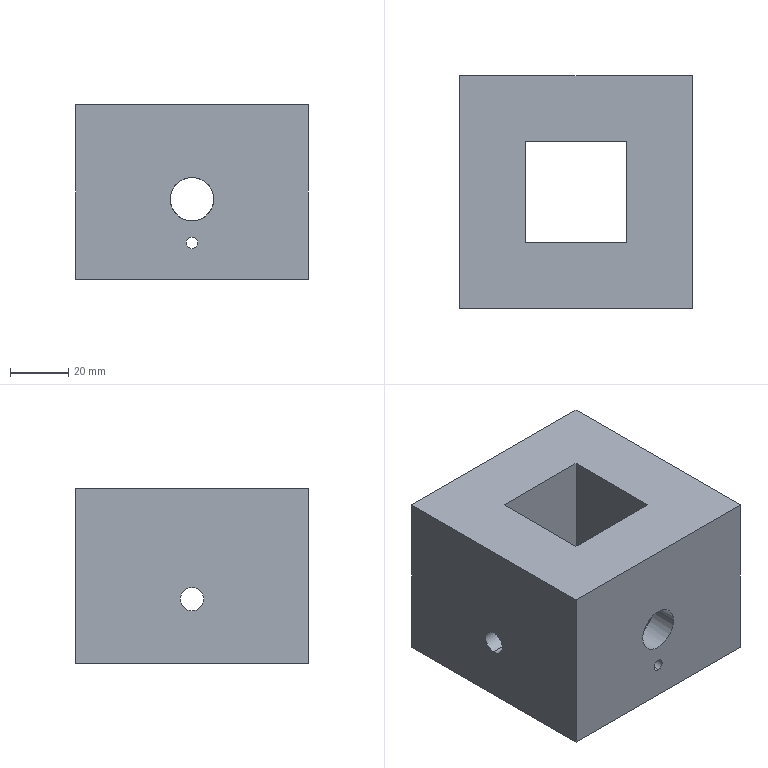Part | SolidWorks | features Cut 6, ICE 3, Extrusion 1 | 1 solid | 43 faces | box 80 x 80 x 60 mm | volume 271765 mm3 | plane 31 | cylinder 12 | commonest cylinder face diameters 4 x4 8 x4 15 x4
STEP:
#1=CARTESIAN_POINT('',(-91.5,-49.,10.5));
#2=VERTEX_POINT('',#1);
#3=CARTESIAN_POINT('',(-91.5,-49.,14.5));
#4=VERTEX_POINT('',#3);
#5=CARTESIAN_POINT('',(-91.5,-49.,12.5));
#6=DIRECTION('',(0.,1.,0.));
#7=DIRECTION('',(0.,0.,-1.));
#8=AXIS2_PLACEMENT_3D('',#5,#6,#7);
#9=CIRCLE('',#8,2.);
#10=EDGE_CURVE('',#2,#4,#9,.T.);
#11=ORIENTED_EDGE('',*,*,#10,.T.);
#12=CARTESIAN_POINT('',(-91.5,-61.5,14.5));
#13=VERTEX_POINT('',#12);
#14=CARTESIAN_POINT('',(-91.5,18.5,14.5));
#15=DIRECTION('',(0.,-1.,0.));
#16=VECTOR('',#15,1000.);
#17=LINE('',#14,#16);
#18=EDGE_CURVE('',#4,#13,#17,.T.);
#19=ORIENTED_EDGE('',*,*,#18,.T.);
#20=CARTESIAN_POINT('',(-91.5,-61.5,10.5));
#21=VERTEX_POINT('',#20);
#22=CARTESIAN_POINT('',(-91.5,-61.5,12.5));
#23=DIRECTION('',(0.,-1.,0.));
#24=DIRECTION('',(-1.,0.,0.));
#25=AXIS2_PLACEMENT_3D('',#22,#23,#24);
#26=CIRCLE('',#25,2.);
#27=EDGE_CURVE('',#13,#21,#26,.T.);
#28=ORIENTED_EDGE('',*,*,#27,.T.);
#29=CARTESIAN_POINT('',(-91.5,18.5,10.5));
#30=DIRECTION('',(0.,-1.,0.));
#31=VECTOR('',#30,1000.);
#32=LINE('',#29,#31);
#33=EDGE_CURVE('',#2,#21,#32,.T.);
#34=ORIENTED_EDGE('',*,*,#33,.F.);
#35=EDGE_LOOP('',(#11,#19,#28,#34));
#36=FACE_OUTER_BOUND('',#35,.T.);
#37=CARTESIAN_POINT('',(-91.5,18.5,12.5));
#38=DIRECTION('',(0.,-1.,0.));
#39=DIRECTION('',(0.,0.,-1.));
#40=AXIS2_PLACEMENT_3D('',#37,#38,#39);
#41=CYLINDRICAL_SURFACE('',#40,2.);
#42=ADVANCED_FACE('',(#36),#41,.F.);
#43=CARTESIAN_POINT('',(-91.5,18.5,10.5));
#44=VERTEX_POINT('',#43);
#45=CARTESIAN_POINT('',(-91.5,18.5,14.5));
#46=VERTEX_POINT('',#45);
#47=CARTESIAN_POINT('',(-91.5,18.5,12.5));
#48=DIRECTION('',(0.,1.,0.));
#49=DIRECTION('',(0.,0.,1.));
#50=AXIS2_PLACEMENT_3D('',#47,#48,#49);
#51=CIRCLE('',#50,2.);
#52=EDGE_CURVE('',#44,#46,#51,.T.);
#53=ORIENTED_EDGE('',*,*,#52,.T.);
#54=CARTESIAN_POINT('',(-91.5,6.,14.5));
#55=VERTEX_POINT('',#54);
#56=CARTESIAN_POINT('',(-91.5,18.5,14.5));
#57=DIRECTION('',(0.,-1.,0.));
#58=VECTOR('',#57,1000.);
#59=LINE('',#56,#58);
#60=EDGE_CURVE('',#46,#55,#59,.T.);
#61=ORIENTED_EDGE('',*,*,#60,.T.);
#62=CARTESIAN_POINT('',(-91.5,6.,10.5));
#63=VERTEX_POINT('',#62);
#64=CARTESIAN_POINT('',(-91.5,6.,12.5));
#65=DIRECTION('',(0.,-1.,0.));
#66=DIRECTION('',(0.,0.,1.));
#67=AXIS2_PLACEMENT_3D('',#64,#65,#66);
#68=CIRCLE('',#67,2.);
#69=EDGE_CURVE('',#55,#63,#68,.T.);
#70=ORIENTED_EDGE('',*,*,#69,.T.);
#71=CARTESIAN_POINT('',(-91.5,18.5,10.5));
#72=DIRECTION('',(0.,-1.,0.));
#73=VECTOR('',#72,1000.);
#74=LINE('',#71,#73);
#75=EDGE_CURVE('',#44,#63,#74,.T.);
#76=ORIENTED_EDGE('',*,*,#75,.F.);
#77=EDGE_LOOP('',(#53,#61,#70,#76));
#78=FACE_OUTER_BOUND('',#77,.T.);
#79=CARTESIAN_POINT('',(-91.5,18.5,12.5));
#80=DIRECTION('',(0.,-1.,0.));
#81=DIRECTION('',(0.,0.,-1.));
#82=AXIS2_PLACEMENT_3D('',#79,#80,#81);
#83=CYLINDRICAL_SURFACE('',#82,2.);
#84=ADVANCED_FACE('',(#78),#83,.F.);
#85=CARTESIAN_POINT('',(-51.5,-21.5,18.));
#86=VERTEX_POINT('',#85);
#87=CARTESIAN_POINT('',(-51.5,-21.5,26.));
#88=VERTEX_POINT('',#87);
#89=CARTESIAN_POINT('',(-51.5,-21.5,22.));
#90=DIRECTION('',(-1.,0.,0.));
#91=DIRECTION('',(0.,0.,1.));
#92=AXIS2_PLACEMENT_3D('',#89,#90,#91);
#93=CIRCLE('',#92,4.);
#94=EDGE_CURVE('',#86,#88,#93,.T.);
#95=ORIENTED_EDGE('',*,*,#94,.F.);
#96=CARTESIAN_POINT('',(-74.,-21.5,18.));
#97=VERTEX_POINT('',#96);
#98=CARTESIAN_POINT('',(-32.5,-21.5,18.));
#99=DIRECTION('',(-1.,0.,0.));
#100=VECTOR('',#99,1000.);
#101=LINE('',#98,#100);
#102=EDGE_CURVE('',#86,#97,#101,.T.);
#103=ORIENTED_EDGE('',*,*,#102,.T.);
#104=CARTESIAN_POINT('',(-74.,-21.5,26.));
#105=VERTEX_POINT('',#104);
#106=CARTESIAN_POINT('',(-74.,-21.5,22.));
#107=DIRECTION('',(1.,0.,0.));
#108=DIRECTION('',(0.,0.,-1.));
#109=AXIS2_PLACEMENT_3D('',#106,#107,#108);
#110=CIRCLE('',#109,4.);
#111=EDGE_CURVE('',#105,#97,#110,.T.);
#112=ORIENTED_EDGE('',*,*,#111,.F.);
#113=CARTESIAN_POINT('',(-32.5,-21.5,26.));
#114=DIRECTION('',(-1.,0.,0.));
#115=VECTOR('',#114,1000.);
#116=LINE('',#113,#115);
#117=EDGE_CURVE('',#88,#105,#116,.T.);
#118=ORIENTED_EDGE('',*,*,#117,.F.);
#119=EDGE_LOOP('',(#95,#103,#112,#118));
#120=FACE_OUTER_BOUND('',#119,.T.);
#121=CARTESIAN_POINT('',(-32.5,-21.5,22.));
#122=DIRECTION('',(-1.,0.,0.));
#123=DIRECTION('',(0.,0.,1.));
#124=AXIS2_PLACEMENT_3D('',#121,#122,#123);
#125=CYLINDRICAL_SURFACE('',#124,4.);
#126=ADVANCED_FACE('',(#120),#125,.F.);
#127=CARTESIAN_POINT('',(-109.,-21.5,18.));
#128=VERTEX_POINT('',#127);
#129=CARTESIAN_POINT('',(-109.,-21.5,26.));
#130=VERTEX_POINT('',#129);
#131=CARTESIAN_POINT('',(-109.,-21.5,22.));
#132=DIRECTION('',(-1.,0.,0.));
#133=DIRECTION('',(0.,0.,1.));
#134=AXIS2_PLACEMENT_3D('',#131,#132,#133);
#135=CIRCLE('',#134,4.);
#136=EDGE_CURVE('',#128,#130,#135,.T.);
#137=ORIENTED_EDGE('',*,*,#136,.F.);
#138=CARTESIAN_POINT('',(-131.5,-21.5,18.));
#139=VERTEX_POINT('',#138);
#140=CARTESIAN_POINT('',(-32.5,-21.5,18.));
#141=DIRECTION('',(-1.,0.,0.));
#142=VECTOR('',#141,1000.);
#143=LINE('',#140,#142);
#144=EDGE_CURVE('',#128,#139,#143,.T.);
#145=ORIENTED_EDGE('',*,*,#144,.T.);
#146=CARTESIAN_POINT('',(-131.5,-21.5,26.));
#147=VERTEX_POINT('',#146);
#148=CARTESIAN_POINT('',(-131.5,-21.5,22.));
#149=DIRECTION('',(-1.,0.,0.));
#150=DIRECTION('',(0.,0.,1.));
#151=AXIS2_PLACEMENT_3D('',#148,#149,#150);
#152=CIRCLE('',#151,4.);
#153=EDGE_CURVE('',#139,#147,#152,.T.);
#154=ORIENTED_EDGE('',*,*,#153,.T.);
#155=CARTESIAN_POINT('',(-32.5,-21.5,26.));
#156=DIRECTION('',(-1.,0.,0.));
#157=VECTOR('',#156,1000.);
#158=LINE('',#155,#157);
#159=EDGE_CURVE('',#130,#147,#158,.T.);
#160=ORIENTED_EDGE('',*,*,#159,.F.);
#161=EDGE_LOOP('',(#137,#145,#154,#160));
#162=FACE_OUTER_BOUND('',#161,.T.);
#163=CARTESIAN_POINT('',(-32.5,-21.5,22.));
#164=DIRECTION('',(-1.,0.,0.));
#165=DIRECTION('',(0.,0.,1.));
#166=AXIS2_PLACEMENT_3D('',#163,#164,#165);
#167=CYLINDRICAL_SURFACE('',#166,4.);
#168=ADVANCED_FACE('',(#162),#167,.F.);
#169=CARTESIAN_POINT('',(-91.5,8.5,20.));
#170=VERTEX_POINT('',#169);
#171=CARTESIAN_POINT('',(-99.,8.5,27.5));
#172=VERTEX_POINT('',#171);
#173=CARTESIAN_POINT('',(-91.5,8.5,27.5));
#174=DIRECTION('',(0.,1.,0.));
#175=DIRECTION('',(0.,0.,1.));
#176=AXIS2_PLACEMENT_3D('',#173,#174,#175);
#177=CIRCLE('',#176,7.5);
#178=EDGE_CURVE('',#170,#172,#177,.T.);
#179=ORIENTED_EDGE('',*,*,#178,.F.);
#180=CARTESIAN_POINT('',(-91.5,18.5,20.));
#181=VERTEX_POINT('',#180);
#182=CARTESIAN_POINT('',(-91.5,8.5,20.));
#183=DIRECTION('',(0.,1.,0.));
#184=VECTOR('',#183,1000.);
#185=LINE('',#182,#184);
#186=EDGE_CURVE('',#170,#181,#185,.T.);
#187=ORIENTED_EDGE('',*,*,#186,.T.);
#188=CARTESIAN_POINT('',(-91.5,18.5,35.));
#189=VERTEX_POINT('',#188);
#190=CARTESIAN_POINT('',(-91.5,18.5,27.5));
#191=DIRECTION('',(0.,1.,0.));
#192=DIRECTION('',(0.,0.,1.));
#193=AXIS2_PLACEMENT_3D('',#190,#191,#192);
#194=CIRCLE('',#193,7.5);
#195=EDGE_CURVE('',#181,#189,#194,.T.);
#196=ORIENTED_EDGE('',*,*,#195,.T.);
#197=CARTESIAN_POINT('',(-91.5,8.5,35.));
#198=VERTEX_POINT('',#197);
#199=CARTESIAN_POINT('',(-91.5,8.5,35.));
#200=DIRECTION('',(0.,1.,0.));
#201=VECTOR('',#200,1000.);
#202=LINE('',#199,#201);
#203=EDGE_CURVE('',#198,#189,#202,.T.);
#204=ORIENTED_EDGE('',*,*,#203,.F.);
#205=CARTESIAN_POINT('',(-91.5,8.5,27.5));
#206=DIRECTION('',(0.,1.,0.));
#207=DIRECTION('',(0.,0.,1.));
#208=AXIS2_PLACEMENT_3D('',#205,#206,#207);
#209=CIRCLE('',#208,7.5);
#210=EDGE_CURVE('',#172,#198,#209,.T.);
#211=ORIENTED_EDGE('',*,*,#210,.F.);
#212=EDGE_LOOP('',(#179,#187,#196,#204,#211));
#213=FACE_OUTER_BOUND('',#212,.T.);
#214=CARTESIAN_POINT('',(-91.5,8.5,27.5));
#215=DIRECTION('',(0.,1.,0.));
#216=DIRECTION('',(0.,0.,1.));
#217=AXIS2_PLACEMENT_3D('',#214,#215,#216);
#218=CYLINDRICAL_SURFACE('',#217,7.5);
#219=ADVANCED_FACE('',(#213),#218,.F.);
#220=CARTESIAN_POINT('',(-99.,-51.5,27.5));
#221=VERTEX_POINT('',#220);
#222=CARTESIAN_POINT('',(-91.5,-51.5,20.));
#223=VERTEX_POINT('',#222);
#224=CARTESIAN_POINT('',(-91.5,-51.5,27.5));
#225=DIRECTION('',(0.,-1.,0.));
#226=DIRECTION('',(1.,0.,0.));
#227=AXIS2_PLACEMENT_3D('',#224,#225,#226);
#228=CIRCLE('',#227,7.5);
#229=EDGE_CURVE('',#221,#223,#228,.T.);
#230=ORIENTED_EDGE('',*,*,#229,.F.);
#231=CARTESIAN_POINT('',(-99.,-61.5,27.5));
#232=VERTEX_POINT('',#231);
#233=CARTESIAN_POINT('',(-99.,-51.5,27.5));
#234=DIRECTION('',(0.,-1.,0.));
#235=VECTOR('',#234,1000.);
#236=LINE('',#233,#235);
#237=EDGE_CURVE('',#221,#232,#236,.T.);
#238=ORIENTED_EDGE('',*,*,#237,.T.);
#239=CARTESIAN_POINT('',(-84.,-61.5,27.5));
#240=VERTEX_POINT('',#239);
#241=CARTESIAN_POINT('',(-91.5,-61.5,27.5));
#242=DIRECTION('',(0.,-1.,0.));
#243=DIRECTION('',(1.,0.,0.));
#244=AXIS2_PLACEMENT_3D('',#241,#242,#243);
#245=CIRCLE('',#244,7.5);
#246=EDGE_CURVE('',#232,#240,#245,.T.);
#247=ORIENTED_EDGE('',*,*,#246,.T.);
#248=CARTESIAN_POINT('',(-84.,-51.5,27.5));
#249=VERTEX_POINT('',#248);
#250=CARTESIAN_POINT('',(-84.,-51.5,27.5));
#251=DIRECTION('',(0.,-1.,0.));
#252=VECTOR('',#251,1000.);
#253=LINE('',#250,#252);
#254=EDGE_CURVE('',#249,#240,#253,.T.);
#255=ORIENTED_EDGE('',*,*,#254,.F.);
#256=CARTESIAN_POINT('',(-91.5,-51.5,27.5));
#257=DIRECTION('',(0.,-1.,0.));
#258=DIRECTION('',(1.,0.,0.));
#259=AXIS2_PLACEMENT_3D('',#256,#257,#258);
#260=CIRCLE('',#259,7.5);
#261=EDGE_CURVE('',#223,#249,#260,.T.);
#262=ORIENTED_EDGE('',*,*,#261,.F.);
#263=EDGE_LOOP('',(#230,#238,#247,#255,#262));
#264=FACE_OUTER_BOUND('',#263,.T.);
#265=CARTESIAN_POINT('',(-91.5,-51.5,27.5));
#266=DIRECTION('',(0.,-1.,0.));
#267=DIRECTION('',(1.,0.,0.));
#268=AXIS2_PLACEMENT_3D('',#265,#266,#267);
#269=CYLINDRICAL_SURFACE('',#268,7.5);
#270=ADVANCED_FACE('',(#264),#269,.F.);
#271=CARTESIAN_POINT('',(-84.,8.5,27.5));
#272=VERTEX_POINT('',#271);
#273=CARTESIAN_POINT('',(-84.,8.5,35.));
#274=VERTEX_POINT('',#273);
#275=CARTESIAN_POINT('',(-84.,8.5,0.));
#276=DIRECTION('',(0.,0.,1.));
#277=VECTOR('',#276,1000.);
#278=LINE('',#275,#277);
#279=EDGE_CURVE('',#272,#274,#278,.T.);
#280=ORIENTED_EDGE('',*,*,#279,.F.);
#281=CARTESIAN_POINT('',(-84.,8.5,20.));
#282=VERTEX_POINT('',#281);
#283=CARTESIAN_POINT('',(-84.,8.5,0.));
#284=DIRECTION('',(0.,0.,1.));
#285=VECTOR('',#284,1000.);
#286=LINE('',#283,#285);
#287=EDGE_CURVE('',#282,#272,#286,.T.);
#288=ORIENTED_EDGE('',*,*,#287,.F.);
#289=CARTESIAN_POINT('',(-84.,-4.,20.));
#290=VERTEX_POINT('',#289);
#291=CARTESIAN_POINT('',(-84.,94.5,20.));
#292=DIRECTION('',(0.,-1.,0.));
#293=VECTOR('',#292,1000.);
#294=LINE('',#291,#293);
#295=EDGE_CURVE('',#282,#290,#294,.T.);
#296=ORIENTED_EDGE('',*,*,#295,.T.);
#297=CARTESIAN_POINT('',(-84.,-4.,35.));
#298=VERTEX_POINT('',#297);
#299=CARTESIAN_POINT('',(-84.,-4.,55.));
#300=DIRECTION('',(0.,0.,-1.));
#301=VECTOR('',#300,1000.);
#302=LINE('',#299,#301);
#303=EDGE_CURVE('',#298,#290,#302,.T.);
#304=ORIENTED_EDGE('',*,*,#303,.F.);
#305=CARTESIAN_POINT('',(-84.,94.5,35.));
#306=DIRECTION('',(0.,-1.,0.));
#307=VECTOR('',#306,1000.);
#308=LINE('',#305,#307);
#309=EDGE_CURVE('',#274,#298,#308,.T.);
#310=ORIENTED_EDGE('',*,*,#309,.F.);
#311=EDGE_LOOP('',(#280,#288,#296,#304,#310));
#312=FACE_OUTER_BOUND('',#311,.T.);
#313=CARTESIAN_POINT('',(-84.,94.5,20.));
#314=DIRECTION('',(1.,0.,0.));
#315=DIRECTION('',(0.,1.,0.));
#316=AXIS2_PLACEMENT_3D('',#313,#314,#315);
#317=PLANE('',#316);
#318=ADVANCED_FACE('',(#312),#317,.F.);
#319=CARTESIAN_POINT('',(0.,8.5,35.));
#320=DIRECTION('',(-1.,0.,0.));
#321=VECTOR('',#320,1000.);
#322=LINE('',#319,#321);
#323=EDGE_CURVE('',#274,#198,#322,.T.);
#324=ORIENTED_EDGE('',*,*,#323,.F.);
#325=ORIENTED_EDGE('',*,*,#309,.T.);
#326=CARTESIAN_POINT('',(-99.,-4.,35.));
#327=VERTEX_POINT('',#326);
#328=CARTESIAN_POINT('',(-74.,-4.,35.));
#329=DIRECTION('',(1.,0.,0.));
#330=VECTOR('',#329,1000.);
#331=LINE('',#328,#330);
#332=EDGE_CURVE('',#327,#298,#331,.T.);
#333=ORIENTED_EDGE('',*,*,#332,.F.);
#334=CARTESIAN_POINT('',(-99.,8.5,35.));
#335=VERTEX_POINT('',#334);
#336=CARTESIAN_POINT('',(-99.,94.5,35.));
#337=DIRECTION('',(0.,-1.,0.));
#338=VECTOR('',#337,1000.);
#339=LINE('',#336,#338);
#340=EDGE_CURVE('',#335,#327,#339,.T.);
#341=ORIENTED_EDGE('',*,*,#340,.F.);
#342=CARTESIAN_POINT('',(0.,8.5,35.));
#343=DIRECTION('',(-1.,0.,0.));
#344=VECTOR('',#343,1000.);
#345=LINE('',#342,#344);
#346=EDGE_CURVE('',#198,#335,#345,.T.);
#347=ORIENTED_EDGE('',*,*,#346,.F.);
#348=EDGE_LOOP('',(#324,#325,#333,#341,#347));
#349=FACE_OUTER_BOUND('',#348,.T.);
#350=CARTESIAN_POINT('',(-84.,94.5,35.));
#351=DIRECTION('',(0.,0.,1.));
#352=DIRECTION('',(1.,0.,0.));
#353=AXIS2_PLACEMENT_3D('',#350,#351,#352);
#354=PLANE('',#353);
#355=ADVANCED_FACE('',(#349),#354,.F.);
#356=CARTESIAN_POINT('',(-99.,8.5,0.));
#357=DIRECTION('',(0.,0.,-1.));
#358=VECTOR('',#357,1000.);
#359=LINE('',#356,#358);
#360=EDGE_CURVE('',#335,#172,#359,.T.);
#361=ORIENTED_EDGE('',*,*,#360,.F.);
#362=ORIENTED_EDGE('',*,*,#340,.T.);
#363=CARTESIAN_POINT('',(-99.,-4.,20.));
#364=VERTEX_POINT('',#363);
#365=CARTESIAN_POINT('',(-99.,-4.,55.));
#366=DIRECTION('',(0.,0.,1.));
#367=VECTOR('',#366,1000.);
#368=LINE('',#365,#367);
#369=EDGE_CURVE('',#364,#327,#368,.T.);
#370=ORIENTED_EDGE('',*,*,#369,.F.);
#371=CARTESIAN_POINT('',(-99.,8.5,20.));
#372=VERTEX_POINT('',#371);
#373=CARTESIAN_POINT('',(-99.,94.5,20.));
#374=DIRECTION('',(0.,-1.,0.));
#375=VECTOR('',#374,1000.);
#376=LINE('',#373,#375);
#377=EDGE_CURVE('',#372,#364,#376,.T.);
#378=ORIENTED_EDGE('',*,*,#377,.F.);
#379=CARTESIAN_POINT('',(-99.,8.5,0.));
#380=DIRECTION('',(0.,0.,-1.));
#381=VECTOR('',#380,1000.);
#382=LINE('',#379,#381);
#383=EDGE_CURVE('',#172,#372,#382,.T.);
#384=ORIENTED_EDGE('',*,*,#383,.F.);
#385=EDGE_LOOP('',(#361,#362,#370,#378,#384));
#386=FACE_OUTER_BOUND('',#385,.T.);
#387=CARTESIAN_POINT('',(-99.,94.5,20.));
#388=DIRECTION('',(-1.,0.,0.));
#389=DIRECTION('',(0.,-1.,0.));
#390=AXIS2_PLACEMENT_3D('',#387,#388,#389);
#391=PLANE('',#390);
#392=ADVANCED_FACE('',(#386),#391,.F.);
#393=CARTESIAN_POINT('',(0.,8.5,20.));
#394=DIRECTION('',(1.,0.,0.));
#395=VECTOR('',#394,1000.);
#396=LINE('',#393,#395);
#397=EDGE_CURVE('',#372,#170,#396,.T.);
#398=ORIENTED_EDGE('',*,*,#397,.F.);
#399=ORIENTED_EDGE('',*,*,#377,.T.);
#400=CARTESIAN_POINT('',(-74.,-4.,20.));
#401=DIRECTION('',(-1.,0.,0.));
#402=VECTOR('',#401,1000.);
#403=LINE('',#400,#402);
#404=EDGE_CURVE('',#290,#364,#403,.T.);
#405=ORIENTED_EDGE('',*,*,#404,.F.);
#406=ORIENTED_EDGE('',*,*,#295,.F.);
#407=CARTESIAN_POINT('',(0.,8.5,20.));
#408=DIRECTION('',(1.,0.,0.));
#409=VECTOR('',#408,1000.);
#410=LINE('',#407,#409);
#411=EDGE_CURVE('',#170,#282,#410,.T.);
#412=ORIENTED_EDGE('',*,*,#411,.F.);
#413=EDGE_LOOP('',(#398,#399,#405,#406,#412));
#414=FACE_OUTER_BOUND('',#413,.T.);
#415=CARTESIAN_POINT('',(-84.,94.5,20.));
#416=DIRECTION('',(0.,0.,-1.));
#417=DIRECTION('',(-1.,0.,0.));
#418=AXIS2_PLACEMENT_3D('',#415,#416,#417);
#419=PLANE('',#418);
#420=ADVANCED_FACE('',(#414),#419,.F.);
#421=CARTESIAN_POINT('',(-99.,-51.5,35.));
#422=VERTEX_POINT('',#421);
#423=CARTESIAN_POINT('',(-99.,-51.5,0.));
#424=DIRECTION('',(0.,0.,1.));
#425=VECTOR('',#424,1000.);
#426=LINE('',#423,#425);
#427=EDGE_CURVE('',#221,#422,#426,.T.);
#428=ORIENTED_EDGE('',*,*,#427,.F.);
#429=CARTESIAN_POINT('',(-99.,-51.5,20.));
#430=VERTEX_POINT('',#429);
#431=CARTESIAN_POINT('',(-99.,-51.5,0.));
#432=DIRECTION('',(0.,0.,1.));
#433=VECTOR('',#432,1000.);
#434=LINE('',#431,#433);
#435=EDGE_CURVE('',#430,#221,#434,.T.);
#436=ORIENTED_EDGE('',*,*,#435,.F.);
#437=CARTESIAN_POINT('',(-99.,-39.,20.));
#438=VERTEX_POINT('',#437);
#439=CARTESIAN_POINT('',(-99.,94.5,20.));
#440=DIRECTION('',(0.,-1.,0.));
#441=VECTOR('',#440,1000.);
#442=LINE('',#439,#441);
#443=EDGE_CURVE('',#438,#430,#442,.T.);
#444=ORIENTED_EDGE('',*,*,#443,.F.);
#445=CARTESIAN_POINT('',(-99.,-39.,35.));
#446=VERTEX_POINT('',#445);
#447=CARTESIAN_POINT('',(-99.,-39.,55.));
#448=DIRECTION('',(0.,0.,-1.));
#449=VECTOR('',#448,1000.);
#450=LINE('',#447,#449);
#451=EDGE_CURVE('',#446,#438,#450,.T.);
#452=ORIENTED_EDGE('',*,*,#451,.F.);
#453=CARTESIAN_POINT('',(-99.,94.5,35.));
#454=DIRECTION('',(0.,-1.,0.));
#455=VECTOR('',#454,1000.);
#456=LINE('',#453,#455);
#457=EDGE_CURVE('',#446,#422,#456,.T.);
#458=ORIENTED_EDGE('',*,*,#457,.T.);
#459=EDGE_LOOP('',(#428,#436,#444,#452,#458));
#460=FACE_OUTER_BOUND('',#459,.T.);
#461=CARTESIAN_POINT('',(-99.,94.5,20.));
#462=DIRECTION('',(-1.,0.,0.));
#463=DIRECTION('',(0.,-1.,0.));
#464=AXIS2_PLACEMENT_3D('',#461,#462,#463);
#465=PLANE('',#464);
#466=ADVANCED_FACE('',(#460),#465,.F.);
#467=CARTESIAN_POINT('',(-91.5,-51.5,35.));
#468=VERTEX_POINT('',#467);
#469=CARTESIAN_POINT('',(0.,-51.5,35.));
#470=DIRECTION('',(1.,0.,0.));
#471=VECTOR('',#470,1000.);
#472=LINE('',#469,#471);
#473=EDGE_CURVE('',#422,#468,#472,.T.);
#474=ORIENTED_EDGE('',*,*,#473,.F.);
#475=ORIENTED_EDGE('',*,*,#457,.F.);
#476=CARTESIAN_POINT('',(-84.,-39.,35.));
#477=VERTEX_POINT('',#476);
#478=CARTESIAN_POINT('',(-74.,-39.,35.));
#479=DIRECTION('',(-1.,0.,0.));
#480=VECTOR('',#479,1000.);
#481=LINE('',#478,#480);
#482=EDGE_CURVE('',#477,#446,#481,.T.);
#483=ORIENTED_EDGE('',*,*,#482,.F.);
#484=CARTESIAN_POINT('',(-84.,-51.5,35.));
#485=VERTEX_POINT('',#484);
#486=CARTESIAN_POINT('',(-84.,94.5,35.));
#487=DIRECTION('',(0.,-1.,0.));
#488=VECTOR('',#487,1000.);
#489=LINE('',#486,#488);
#490=EDGE_CURVE('',#477,#485,#489,.T.);
#491=ORIENTED_EDGE('',*,*,#490,.T.);
#492=CARTESIAN_POINT('',(0.,-51.5,35.));
#493=DIRECTION('',(1.,0.,0.));
#494=VECTOR('',#493,1000.);
#495=LINE('',#492,#494);
#496=EDGE_CURVE('',#468,#485,#495,.T.);
#497=ORIENTED_EDGE('',*,*,#496,.F.);
#498=EDGE_LOOP('',(#474,#475,#483,#491,#497));
#499=FACE_OUTER_BOUND('',#498,.T.);
#500=CARTESIAN_POINT('',(-84.,94.5,35.));
#501=DIRECTION('',(0.,0.,1.));
#502=DIRECTION('',(1.,0.,0.));
#503=AXIS2_PLACEMENT_3D('',#500,#501,#502);
#504=PLANE('',#503);
#505=ADVANCED_FACE('',(#499),#504,.F.);
#506=CARTESIAN_POINT('',(-84.,-51.5,0.));
#507=DIRECTION('',(0.,0.,-1.));
#508=VECTOR('',#507,1000.);
#509=LINE('',#506,#508);
#510=EDGE_CURVE('',#485,#249,#509,.T.);
#511=ORIENTED_EDGE('',*,*,#510,.F.);
#512=ORIENTED_EDGE('',*,*,#490,.F.);
#513=CARTESIAN_POINT('',(-84.,-39.,20.));
#514=VERTEX_POINT('',#513);
#515=CARTESIAN_POINT('',(-84.,-39.,55.));
#516=DIRECTION('',(0.,0.,1.));
#517=VECTOR('',#516,1000.);
#518=LINE('',#515,#517);
#519=EDGE_CURVE('',#514,#477,#518,.T.);
#520=ORIENTED_EDGE('',*,*,#519,.F.);
#521=CARTESIAN_POINT('',(-84.,-51.5,20.));
#522=VERTEX_POINT('',#521);
#523=CARTESIAN_POINT('',(-84.,94.5,20.));
#524=DIRECTION('',(0.,-1.,0.));
#525=VECTOR('',#524,1000.);
#526=LINE('',#523,#525);
#527=EDGE_CURVE('',#514,#522,#526,.T.);
#528=ORIENTED_EDGE('',*,*,#527,.T.);
#529=CARTESIAN_POINT('',(-84.,-51.5,0.));
#530=DIRECTION('',(0.,0.,-1.));
#531=VECTOR('',#530,1000.);
#532=LINE('',#529,#531);
#533=EDGE_CURVE('',#249,#522,#532,.T.);
#534=ORIENTED_EDGE('',*,*,#533,.F.);
#535=EDGE_LOOP('',(#511,#512,#520,#528,#534));
#536=FACE_OUTER_BOUND('',#535,.T.);
#537=CARTESIAN_POINT('',(-84.,94.5,20.));
#538=DIRECTION('',(1.,0.,0.));
#539=DIRECTION('',(0.,1.,0.));
#540=AXIS2_PLACEMENT_3D('',#537,#538,#539);
#541=PLANE('',#540);
#542=ADVANCED_FACE('',(#536),#541,.F.);
#543=CARTESIAN_POINT('',(0.,-51.5,20.));
#544=DIRECTION('',(-1.,0.,0.));
#545=VECTOR('',#544,1000.);
#546=LINE('',#543,#545);
#547=EDGE_CURVE('',#522,#223,#546,.T.);
#548=ORIENTED_EDGE('',*,*,#547,.F.);
#549=ORIENTED_EDGE('',*,*,#527,.F.);
#550=CARTESIAN_POINT('',(-74.,-39.,20.));
#551=DIRECTION('',(1.,0.,0.));
#552=VECTOR('',#551,1000.);
#553=LINE('',#550,#552);
#554=EDGE_CURVE('',#438,#514,#553,.T.);
#555=ORIENTED_EDGE('',*,*,#554,.F.);
#556=ORIENTED_EDGE('',*,*,#443,.T.);
#557=CARTESIAN_POINT('',(0.,-51.5,20.));
#558=DIRECTION('',(-1.,0.,0.));
#559=VECTOR('',#558,1000.);
#560=LINE('',#557,#559);
#561=EDGE_CURVE('',#223,#430,#560,.T.);
#562=ORIENTED_EDGE('',*,*,#561,.F.);
#563=EDGE_LOOP('',(#548,#549,#555,#556,#562));
#564=FACE_OUTER_BOUND('',#563,.T.);
#565=CARTESIAN_POINT('',(-84.,94.5,20.));
#566=DIRECTION('',(0.,0.,-1.));
#567=DIRECTION('',(-1.,0.,0.));
#568=AXIS2_PLACEMENT_3D('',#565,#566,#567);
#569=PLANE('',#568);
#570=ADVANCED_FACE('',(#564),#569,.F.);
#571=CARTESIAN_POINT('',(-131.5,-21.5,22.));
#572=DIRECTION('',(-1.,0.,0.));
#573=DIRECTION('',(0.,0.,1.));
#574=AXIS2_PLACEMENT_3D('',#571,#572,#573);
#575=CIRCLE('',#574,4.);
#576=EDGE_CURVE('',#147,#139,#575,.T.);
#577=ORIENTED_EDGE('',*,*,#576,.F.);
#578=ORIENTED_EDGE('',*,*,#153,.F.);
#579=EDGE_LOOP('',(#577,#578));
#580=FACE_BOUND('',#579,.T.);
#581=CARTESIAN_POINT('',(-131.5,18.5,60.));
#582=VERTEX_POINT('',#581);
#583=CARTESIAN_POINT('',(-131.5,18.5,0.));
#584=VERTEX_POINT('',#583);
#585=CARTESIAN_POINT('',(-131.5,18.5,60.));
#586=DIRECTION('',(0.,0.,-1.));
#587=VECTOR('',#586,1000.);
#588=LINE('',#585,#587);
#589=EDGE_CURVE('',#582,#584,#588,.T.);
#590=ORIENTED_EDGE('',*,*,#589,.T.);
#591=CARTESIAN_POINT('',(-131.5,-61.5,0.));
#592=VERTEX_POINT('',#591);
#593=CARTESIAN_POINT('',(-131.5,-61.5,0.));
#594=DIRECTION('',(0.,1.,0.));
#595=VECTOR('',#594,1000.);
#596=LINE('',#593,#595);
#597=EDGE_CURVE('',#592,#584,#596,.T.);
#598=ORIENTED_EDGE('',*,*,#597,.F.);
#599=CARTESIAN_POINT('',(-131.5,-61.5,60.));
#600=VERTEX_POINT('',#599);
#601=CARTESIAN_POINT('',(-131.5,-61.5,60.));
#602=DIRECTION('',(0.,0.,-1.));
#603=VECTOR('',#602,1000.);
#604=LINE('',#601,#603);
#605=EDGE_CURVE('',#600,#592,#604,.T.);
#606=ORIENTED_EDGE('',*,*,#605,.F.);
#607=CARTESIAN_POINT('',(-131.5,-61.5,60.));
#608=DIRECTION('',(0.,-1.,0.));
#609=VECTOR('',#608,1000.);
#610=LINE('',#607,#609);
#611=EDGE_CURVE('',#582,#600,#610,.T.);
#612=ORIENTED_EDGE('',*,*,#611,.F.);
#613=EDGE_LOOP('',(#590,#598,#606,#612));
#614=FACE_OUTER_BOUND('',#613,.T.);
#615=CARTESIAN_POINT('',(-131.5,-61.5,60.));
#616=DIRECTION('',(1.,0.,0.));
#617=DIRECTION('',(0.,0.,-1.));
#618=AXIS2_PLACEMENT_3D('',#615,#616,#617);
#619=PLANE('',#618);
#620=ADVANCED_FACE('',(#580,#614),#619,.F.);
#621=CARTESIAN_POINT('',(-91.5,-61.5,12.5));
#622=DIRECTION('',(0.,-1.,0.));
#623=DIRECTION('',(-1.,0.,0.));
#624=AXIS2_PLACEMENT_3D('',#621,#622,#623);
#625=CIRCLE('',#624,2.);
#626=EDGE_CURVE('',#21,#13,#625,.T.);
#627=ORIENTED_EDGE('',*,*,#626,.F.);
#628=ORIENTED_EDGE('',*,*,#27,.F.);
#629=EDGE_LOOP('',(#627,#628));
#630=FACE_BOUND('',#629,.T.);
#631=CARTESIAN_POINT('',(-91.5,-61.5,27.5));
#632=DIRECTION('',(0.,-1.,0.));
#633=DIRECTION('',(1.,0.,0.));
#634=AXIS2_PLACEMENT_3D('',#631,#632,#633);
#635=CIRCLE('',#634,7.5);
#636=EDGE_CURVE('',#240,#232,#635,.T.);
#637=ORIENTED_EDGE('',*,*,#636,.F.);
#638=ORIENTED_EDGE('',*,*,#246,.F.);
#639=EDGE_LOOP('',(#637,#638));
#640=FACE_BOUND('',#639,.T.);
#641=ORIENTED_EDGE('',*,*,#605,.T.);
#642=CARTESIAN_POINT('',(-51.5,-61.5,0.));
#643=VERTEX_POINT('',#642);
#644=CARTESIAN_POINT('',(-51.5,-61.5,0.));
#645=DIRECTION('',(-1.,0.,0.));
#646=VECTOR('',#645,1000.);
#647=LINE('',#644,#646);
#648=EDGE_CURVE('',#643,#592,#647,.T.);
#649=ORIENTED_EDGE('',*,*,#648,.F.);
#650=CARTESIAN_POINT('',(-51.5,-61.5,60.));
#651=VERTEX_POINT('',#650);
#652=CARTESIAN_POINT('',(-51.5,-61.5,60.));
#653=DIRECTION('',(0.,0.,-1.));
#654=VECTOR('',#653,1000.);
#655=LINE('',#652,#654);
#656=EDGE_CURVE('',#651,#643,#655,.T.);
#657=ORIENTED_EDGE('',*,*,#656,.F.);
#658=CARTESIAN_POINT('',(-51.5,-61.5,60.));
#659=DIRECTION('',(1.,0.,0.));
#660=VECTOR('',#659,1000.);
#661=LINE('',#658,#660);
#662=EDGE_CURVE('',#600,#651,#661,.T.);
#663=ORIENTED_EDGE('',*,*,#662,.F.);
#664=EDGE_LOOP('',(#641,#649,#657,#663));
#665=FACE_OUTER_BOUND('',#664,.T.);
#666=CARTESIAN_POINT('',(-51.5,-61.5,60.));
#667=DIRECTION('',(0.,1.,0.));
#668=DIRECTION('',(-1.,0.,0.));
#669=AXIS2_PLACEMENT_3D('',#666,#667,#668);
#670=PLANE('',#669);
#671=ADVANCED_FACE('',(#630,#640,#665),#670,.F.);
#672=CARTESIAN_POINT('',(-51.5,-21.5,22.));
#673=DIRECTION('',(-1.,0.,0.));
#674=DIRECTION('',(0.,0.,1.));
#675=AXIS2_PLACEMENT_3D('',#672,#673,#674);
#676=CIRCLE('',#675,4.);
#677=EDGE_CURVE('',#88,#86,#676,.T.);
#678=ORIENTED_EDGE('',*,*,#677,.T.);
#679=ORIENTED_EDGE('',*,*,#94,.T.);
#680=EDGE_LOOP('',(#678,#679));
#681=FACE_BOUND('',#680,.T.);
#682=ORIENTED_EDGE('',*,*,#656,.T.);
#683=CARTESIAN_POINT('',(-51.5,18.5,0.));
#684=VERTEX_POINT('',#683);
#685=CARTESIAN_POINT('',(-51.5,18.5,0.));
#686=DIRECTION('',(0.,-1.,0.));
#687=VECTOR('',#686,1000.);
#688=LINE('',#685,#687);
#689=EDGE_CURVE('',#684,#643,#688,.T.);
#690=ORIENTED_EDGE('',*,*,#689,.F.);
#691=CARTESIAN_POINT('',(-51.5,18.5,60.));
#692=VERTEX_POINT('',#691);
#693=CARTESIAN_POINT('',(-51.5,18.5,60.));
#694=DIRECTION('',(0.,0.,-1.));
#695=VECTOR('',#694,1000.);
#696=LINE('',#693,#695);
#697=EDGE_CURVE('',#692,#684,#696,.T.);
#698=ORIENTED_EDGE('',*,*,#697,.F.);
#699=CARTESIAN_POINT('',(-51.5,-61.5,60.));
#700=DIRECTION('',(0.,1.,0.));
#701=VECTOR('',#700,1000.);
#702=LINE('',#699,#701);
#703=EDGE_CURVE('',#651,#692,#702,.T.);
#704=ORIENTED_EDGE('',*,*,#703,.F.);
#705=EDGE_LOOP('',(#682,#690,#698,#704));
#706=FACE_OUTER_BOUND('',#705,.T.);
#707=CARTESIAN_POINT('',(-51.5,-61.5,60.));
#708=DIRECTION('',(-1.,0.,0.));
#709=DIRECTION('',(0.,0.,1.));
#710=AXIS2_PLACEMENT_3D('',#707,#708,#709);
#711=PLANE('',#710);
#712=ADVANCED_FACE('',(#681,#706),#711,.F.);
#713=ORIENTED_EDGE('',*,*,#52,.F.);
#714=CARTESIAN_POINT('',(-91.5,18.5,12.5));
#715=DIRECTION('',(0.,1.,0.));
#716=DIRECTION('',(0.,0.,1.));
#717=AXIS2_PLACEMENT_3D('',#714,#715,#716);
#718=CIRCLE('',#717,2.);
#719=EDGE_CURVE('',#46,#44,#718,.T.);
#720=ORIENTED_EDGE('',*,*,#719,.F.);
#721=EDGE_LOOP('',(#713,#720));
#722=FACE_BOUND('',#721,.T.);
#723=CARTESIAN_POINT('',(-91.5,18.5,27.5));
#724=DIRECTION('',(0.,1.,0.));
#725=DIRECTION('',(0.,0.,1.));
#726=AXIS2_PLACEMENT_3D('',#723,#724,#725);
#727=CIRCLE('',#726,7.5);
#728=EDGE_CURVE('',#189,#181,#727,.T.);
#729=ORIENTED_EDGE('',*,*,#728,.F.);
#730=ORIENTED_EDGE('',*,*,#195,.F.);
#731=EDGE_LOOP('',(#729,#730));
#732=FACE_BOUND('',#731,.T.);
#733=ORIENTED_EDGE('',*,*,#697,.T.);
#734=CARTESIAN_POINT('',(-131.5,18.5,0.));
#735=DIRECTION('',(1.,0.,0.));
#736=VECTOR('',#735,1000.);
#737=LINE('',#734,#736);
#738=EDGE_CURVE('',#584,#684,#737,.T.);
#739=ORIENTED_EDGE('',*,*,#738,.F.);
#740=ORIENTED_EDGE('',*,*,#589,.F.);
#741=CARTESIAN_POINT('',(-51.5,18.5,60.));
#742=DIRECTION('',(-1.,0.,0.));
#743=VECTOR('',#742,1000.);
#744=LINE('',#741,#743);
#745=EDGE_CURVE('',#692,#582,#744,.T.);
#746=ORIENTED_EDGE('',*,*,#745,.F.);
#747=EDGE_LOOP('',(#733,#739,#740,#746));
#748=FACE_OUTER_BOUND('',#747,.T.);
#749=CARTESIAN_POINT('',(-51.5,18.5,60.));
#750=DIRECTION('',(0.,-1.,0.));
#751=DIRECTION('',(0.,0.,-1.));
#752=AXIS2_PLACEMENT_3D('',#749,#750,#751);
#753=PLANE('',#752);
#754=ADVANCED_FACE('',(#722,#732,#748),#753,.F.);
#755=CARTESIAN_POINT('',(-109.,-39.,60.));
#756=VERTEX_POINT('',#755);
#757=CARTESIAN_POINT('',(-74.,-39.,60.));
#758=VERTEX_POINT('',#757);
#759=CARTESIAN_POINT('',(0.,-39.,60.));
#760=DIRECTION('',(1.,0.,0.));
#761=VECTOR('',#760,1000.);
#762=LINE('',#759,#761);
#763=EDGE_CURVE('',#756,#758,#762,.T.);
#764=ORIENTED_EDGE('',*,*,#763,.F.);
#765=CARTESIAN_POINT('',(-109.,-4.,60.));
#766=VERTEX_POINT('',#765);
#767=CARTESIAN_POINT('',(-109.,0.,60.));
#768=DIRECTION('',(0.,-1.,0.));
#769=VECTOR('',#768,1000.);
#770=LINE('',#767,#769);
#771=EDGE_CURVE('',#766,#756,#770,.T.);
#772=ORIENTED_EDGE('',*,*,#771,.F.);
#773=CARTESIAN_POINT('',(-74.,-4.,60.));
#774=VERTEX_POINT('',#773);
#775=CARTESIAN_POINT('',(0.,-4.,60.));
#776=DIRECTION('',(-1.,0.,0.));
#777=VECTOR('',#776,1000.);
#778=LINE('',#775,#777);
#779=EDGE_CURVE('',#774,#766,#778,.T.);
#780=ORIENTED_EDGE('',*,*,#779,.F.);
#781=CARTESIAN_POINT('',(-74.,0.,60.));
#782=DIRECTION('',(0.,1.,0.));
#783=VECTOR('',#782,1000.);
#784=LINE('',#781,#783);
#785=EDGE_CURVE('',#758,#774,#784,.T.);
#786=ORIENTED_EDGE('',*,*,#785,.F.);
#787=EDGE_LOOP('',(#764,#772,#780,#786));
#788=FACE_BOUND('',#787,.T.);
#789=ORIENTED_EDGE('',*,*,#611,.T.);
#790=ORIENTED_EDGE('',*,*,#662,.T.);
#791=ORIENTED_EDGE('',*,*,#703,.T.);
#792=ORIENTED_EDGE('',*,*,#745,.T.);
#793=EDGE_LOOP('',(#789,#790,#791,#792));
#794=FACE_OUTER_BOUND('',#793,.T.);
#795=CARTESIAN_POINT('',(0.,0.,60.));
#796=DIRECTION('',(0.,0.,1.));
#797=DIRECTION('',(1.,0.,0.));
#798=AXIS2_PLACEMENT_3D('',#795,#796,#797);
#799=PLANE('',#798);
#800=ADVANCED_FACE('',(#788,#794),#799,.T.);
#801=CARTESIAN_POINT('',(-64.,-49.,15.));
#802=VERTEX_POINT('',#801);
#803=CARTESIAN_POINT('',(-119.,-49.,15.));
#804=VERTEX_POINT('',#803);
#805=CARTESIAN_POINT('',(-64.,-49.,15.));
#806=DIRECTION('',(-1.,0.,0.));
#807=VECTOR('',#806,1000.);
#808=LINE('',#805,#807);
#809=EDGE_CURVE('',#802,#804,#808,.T.);
#810=ORIENTED_EDGE('',*,*,#809,.T.);
#811=CARTESIAN_POINT('',(-119.,6.,15.));
#812=VERTEX_POINT('',#811);
#813=CARTESIAN_POINT('',(-119.,-49.,15.));
#814=DIRECTION('',(0.,1.,0.));
#815=VECTOR('',#814,1000.);
#816=LINE('',#813,#815);
#817=EDGE_CURVE('',#804,#812,#816,.T.);
#818=ORIENTED_EDGE('',*,*,#817,.T.);
#819=CARTESIAN_POINT('',(-64.,6.,15.));
#820=VERTEX_POINT('',#819);
#821=CARTESIAN_POINT('',(-119.,6.,15.));
#822=DIRECTION('',(1.,0.,0.));
#823=VECTOR('',#822,1000.);
#824=LINE('',#821,#823);
#825=EDGE_CURVE('',#812,#820,#824,.T.);
#826=ORIENTED_EDGE('',*,*,#825,.T.);
#827=CARTESIAN_POINT('',(-64.,6.,15.));
#828=DIRECTION('',(0.,-1.,0.));
#829=VECTOR('',#828,1000.);
#830=LINE('',#827,#829);
#831=EDGE_CURVE('',#820,#802,#830,.T.);
#832=ORIENTED_EDGE('',*,*,#831,.T.);
#833=EDGE_LOOP('',(#810,#818,#826,#832));
#834=FACE_OUTER_BOUND('',#833,.T.);
#835=CARTESIAN_POINT('',(-109.,-4.,15.));
#836=VERTEX_POINT('',#835);
#837=CARTESIAN_POINT('',(-109.,-39.,15.));
#838=VERTEX_POINT('',#837);
#839=CARTESIAN_POINT('',(-109.,-4.,15.));
#840=DIRECTION('',(0.,-1.,0.));
#841=VECTOR('',#840,1000.);
#842=LINE('',#839,#841);
#843=EDGE_CURVE('',#836,#838,#842,.T.);
#844=ORIENTED_EDGE('',*,*,#843,.T.);
#845=CARTESIAN_POINT('',(-74.,-39.,15.));
#846=VERTEX_POINT('',#845);
#847=CARTESIAN_POINT('',(-74.,-39.,15.));
#848=DIRECTION('',(1.,0.,0.));
#849=VECTOR('',#848,1000.);
#850=LINE('',#847,#849);
#851=EDGE_CURVE('',#838,#846,#850,.T.);
#852=ORIENTED_EDGE('',*,*,#851,.T.);
#853=CARTESIAN_POINT('',(-74.,-4.,15.));
#854=VERTEX_POINT('',#853);
#855=CARTESIAN_POINT('',(-74.,-4.,15.));
#856=DIRECTION('',(0.,1.,0.));
#857=VECTOR('',#856,1000.);
#858=LINE('',#855,#857);
#859=EDGE_CURVE('',#846,#854,#858,.T.);
#860=ORIENTED_EDGE('',*,*,#859,.T.);
#861=CARTESIAN_POINT('',(-74.,-4.,15.));
#862=DIRECTION('',(-1.,0.,0.));
#863=VECTOR('',#862,1000.);
#864=LINE('',#861,#863);
#865=EDGE_CURVE('',#854,#836,#864,.T.);
#866=ORIENTED_EDGE('',*,*,#865,.T.);
#867=EDGE_LOOP('',(#844,#852,#860,#866));
#868=FACE_BOUND('',#867,.T.);
#869=CARTESIAN_POINT('',(0.,0.,15.));
#870=DIRECTION('',(0.,0.,-1.));
#871=DIRECTION('',(-1.,0.,0.));
#872=AXIS2_PLACEMENT_3D('',#869,#870,#871);
#873=PLANE('',#872);
#874=ADVANCED_FACE('',(#834,#868),#873,.T.);
#875=ORIENTED_EDGE('',*,*,#10,.F.);
#876=CARTESIAN_POINT('',(-91.5,-49.,12.5));
#877=DIRECTION('',(0.,1.,0.));
#878=DIRECTION('',(0.,0.,-1.));
#879=AXIS2_PLACEMENT_3D('',#876,#877,#878);
#880=CIRCLE('',#879,2.);
#881=EDGE_CURVE('',#4,#2,#880,.T.);
#882=ORIENTED_EDGE('',*,*,#881,.F.);
#883=EDGE_LOOP('',(#875,#882));
#884=FACE_BOUND('',#883,.T.);
#885=CARTESIAN_POINT('',(-64.,-49.,0.));
#886=VERTEX_POINT('',#885);
#887=CARTESIAN_POINT('',(-64.,-49.,15.));
#888=DIRECTION('',(0.,0.,-1.));
#889=VECTOR('',#888,1000.);
#890=LINE('',#887,#889);
#891=EDGE_CURVE('',#802,#886,#890,.T.);
#892=ORIENTED_EDGE('',*,*,#891,.T.);
#893=CARTESIAN_POINT('',(-119.,-49.,0.));
#894=VERTEX_POINT('',#893);
#895=CARTESIAN_POINT('',(-64.,-49.,0.));
#896=DIRECTION('',(-1.,0.,0.));
#897=VECTOR('',#896,1000.);
#898=LINE('',#895,#897);
#899=EDGE_CURVE('',#886,#894,#898,.T.);
#900=ORIENTED_EDGE('',*,*,#899,.T.);
#901=CARTESIAN_POINT('',(-119.,-49.,15.));
#902=DIRECTION('',(0.,0.,-1.));
#903=VECTOR('',#902,1000.);
#904=LINE('',#901,#903);
#905=EDGE_CURVE('',#804,#894,#904,.T.);
#906=ORIENTED_EDGE('',*,*,#905,.F.);
#907=ORIENTED_EDGE('',*,*,#809,.F.);
#908=EDGE_LOOP('',(#892,#900,#906,#907));
#909=FACE_OUTER_BOUND('',#908,.T.);
#910=CARTESIAN_POINT('',(-64.,-49.,15.));
#911=DIRECTION('',(0.,-1.,0.));
#912=DIRECTION('',(0.,0.,-1.));
#913=AXIS2_PLACEMENT_3D('',#910,#911,#912);
#914=PLANE('',#913);
#915=ADVANCED_FACE('',(#884,#909),#914,.F.);
#916=CARTESIAN_POINT('',(-64.,6.,0.));
#917=VERTEX_POINT('',#916);
#918=CARTESIAN_POINT('',(-64.,6.,15.));
#919=DIRECTION('',(0.,0.,-1.));
#920=VECTOR('',#919,1000.);
#921=LINE('',#918,#920);
#922=EDGE_CURVE('',#820,#917,#921,.T.);
#923=ORIENTED_EDGE('',*,*,#922,.T.);
#924=CARTESIAN_POINT('',(-64.,6.,0.));
#925=DIRECTION('',(0.,-1.,0.));
#926=VECTOR('',#925,1000.);
#927=LINE('',#924,#926);
#928=EDGE_CURVE('',#917,#886,#927,.T.);
#929=ORIENTED_EDGE('',*,*,#928,.T.);
#930=ORIENTED_EDGE('',*,*,#891,.F.);
#931=ORIENTED_EDGE('',*,*,#831,.F.);
#932=EDGE_LOOP('',(#923,#929,#930,#931));
#933=FACE_OUTER_BOUND('',#932,.T.);
#934=CARTESIAN_POINT('',(-64.,6.,15.));
#935=DIRECTION('',(1.,0.,0.));
#936=DIRECTION('',(0.,0.,-1.));
#937=AXIS2_PLACEMENT_3D('',#934,#935,#936);
#938=PLANE('',#937);
#939=ADVANCED_FACE('',(#933),#938,.F.);
#940=CARTESIAN_POINT('',(-91.5,6.,12.5));
#941=DIRECTION('',(0.,-1.,0.));
#942=DIRECTION('',(0.,0.,1.));
#943=AXIS2_PLACEMENT_3D('',#940,#941,#942);
#944=CIRCLE('',#943,2.);
#945=EDGE_CURVE('',#63,#55,#944,.T.);
#946=ORIENTED_EDGE('',*,*,#945,.F.);
#947=ORIENTED_EDGE('',*,*,#69,.F.);
#948=EDGE_LOOP('',(#946,#947));
#949=FACE_BOUND('',#948,.T.);
#950=CARTESIAN_POINT('',(-119.,6.,0.));
#951=VERTEX_POINT('',#950);
#952=CARTESIAN_POINT('',(-119.,6.,15.));
#953=DIRECTION('',(0.,0.,-1.));
#954=VECTOR('',#953,1000.);
#955=LINE('',#952,#954);
#956=EDGE_CURVE('',#812,#951,#955,.T.);
#957=ORIENTED_EDGE('',*,*,#956,.T.);
#958=CARTESIAN_POINT('',(-119.,6.,0.));
#959=DIRECTION('',(1.,0.,0.));
#960=VECTOR('',#959,1000.);
#961=LINE('',#958,#960);
#962=EDGE_CURVE('',#951,#917,#961,.T.);
#963=ORIENTED_EDGE('',*,*,#962,.T.);
#964=ORIENTED_EDGE('',*,*,#922,.F.);
#965=ORIENTED_EDGE('',*,*,#825,.F.);
#966=EDGE_LOOP('',(#957,#963,#964,#965));
#967=FACE_OUTER_BOUND('',#966,.T.);
#968=CARTESIAN_POINT('',(-119.,6.,15.));
#969=DIRECTION('',(0.,1.,0.));
#970=DIRECTION('',(0.,0.,1.));
#971=AXIS2_PLACEMENT_3D('',#968,#969,#970);
#972=PLANE('',#971);
#973=ADVANCED_FACE('',(#949,#967),#972,.F.);
#974=ORIENTED_EDGE('',*,*,#905,.T.);
#975=CARTESIAN_POINT('',(-119.,-49.,0.));
#976=DIRECTION('',(0.,1.,0.));
#977=VECTOR('',#976,1000.);
#978=LINE('',#975,#977);
#979=EDGE_CURVE('',#894,#951,#978,.T.);
#980=ORIENTED_EDGE('',*,*,#979,.T.);
#981=ORIENTED_EDGE('',*,*,#956,.F.);
#982=ORIENTED_EDGE('',*,*,#817,.F.);
#983=EDGE_LOOP('',(#974,#980,#981,#982));
#984=FACE_OUTER_BOUND('',#983,.T.);
#985=CARTESIAN_POINT('',(-119.,-49.,15.));
#986=DIRECTION('',(-1.,0.,0.));
#987=DIRECTION('',(0.,0.,1.));
#988=AXIS2_PLACEMENT_3D('',#985,#986,#987);
#989=PLANE('',#988);
#990=ADVANCED_FACE('',(#984),#989,.F.);
#991=ORIENTED_EDGE('',*,*,#404,.T.);
#992=ORIENTED_EDGE('',*,*,#369,.T.);
#993=ORIENTED_EDGE('',*,*,#332,.T.);
#994=ORIENTED_EDGE('',*,*,#303,.T.);
#995=EDGE_LOOP('',(#991,#992,#993,#994));
#996=FACE_BOUND('',#995,.T.);
#997=ORIENTED_EDGE('',*,*,#865,.F.);
#998=CARTESIAN_POINT('',(-74.,-4.,55.));
#999=DIRECTION('',(0.,0.,-1.));
#1000=VECTOR('',#999,1000.);
#1001=LINE('',#998,#1000);
#1002=EDGE_CURVE('',#774,#854,#1001,.T.);
#1003=ORIENTED_EDGE('',*,*,#1002,.F.);
#1004=ORIENTED_EDGE('',*,*,#779,.T.);
#1005=CARTESIAN_POINT('',(-109.,-4.,55.));
#1006=DIRECTION('',(0.,0.,-1.));
#1007=VECTOR('',#1006,1000.);
#1008=LINE('',#1005,#1007);
#1009=EDGE_CURVE('',#766,#836,#1008,.T.);
#1010=ORIENTED_EDGE('',*,*,#1009,.T.);
#1011=EDGE_LOOP('',(#997,#1003,#1004,#1010));
#1012=FACE_OUTER_BOUND('',#1011,.T.);
#1013=CARTESIAN_POINT('',(-74.,-4.,55.));
#1014=DIRECTION('',(0.,1.,0.));
#1015=DIRECTION('',(0.,0.,1.));
#1016=AXIS2_PLACEMENT_3D('',#1013,#1014,#1015);
#1017=PLANE('',#1016);
#1018=ADVANCED_FACE('',(#996,#1012),#1017,.F.);
#1019=ORIENTED_EDGE('',*,*,#111,.T.);
#1020=CARTESIAN_POINT('',(-74.,-21.5,22.));
#1021=DIRECTION('',(1.,0.,0.));
#1022=DIRECTION('',(0.,0.,-1.));
#1023=AXIS2_PLACEMENT_3D('',#1020,#1021,#1022);
#1024=CIRCLE('',#1023,4.);
#1025=EDGE_CURVE('',#97,#105,#1024,.T.);
#1026=ORIENTED_EDGE('',*,*,#1025,.T.);
#1027=EDGE_LOOP('',(#1019,#1026));
#1028=FACE_BOUND('',#1027,.T.);
#1029=ORIENTED_EDGE('',*,*,#859,.F.);
#1030=CARTESIAN_POINT('',(-74.,-39.,55.));
#1031=DIRECTION('',(0.,0.,-1.));
#1032=VECTOR('',#1031,1000.);
#1033=LINE('',#1030,#1032);
#1034=EDGE_CURVE('',#758,#846,#1033,.T.);
#1035=ORIENTED_EDGE('',*,*,#1034,.F.);
#1036=ORIENTED_EDGE('',*,*,#785,.T.);
#1037=ORIENTED_EDGE('',*,*,#1002,.T.);
#1038=EDGE_LOOP('',(#1029,#1035,#1036,#1037));
#1039=FACE_OUTER_BOUND('',#1038,.T.);
#1040=CARTESIAN_POINT('',(-74.,-4.,55.));
#1041=DIRECTION('',(1.,0.,0.));
#1042=DIRECTION('',(0.,0.,-1.));
#1043=AXIS2_PLACEMENT_3D('',#1040,#1041,#1042);
#1044=PLANE('',#1043);
#1045=ADVANCED_FACE('',(#1028,#1039),#1044,.F.);
#1046=ORIENTED_EDGE('',*,*,#482,.T.);
#1047=ORIENTED_EDGE('',*,*,#451,.T.);
#1048=ORIENTED_EDGE('',*,*,#554,.T.);
#1049=ORIENTED_EDGE('',*,*,#519,.T.);
#1050=EDGE_LOOP('',(#1046,#1047,#1048,#1049));
#1051=FACE_BOUND('',#1050,.T.);
#1052=ORIENTED_EDGE('',*,*,#851,.F.);
#1053=CARTESIAN_POINT('',(-109.,-39.,55.));
#1054=DIRECTION('',(0.,0.,-1.));
#1055=VECTOR('',#1054,1000.);
#1056=LINE('',#1053,#1055);
#1057=EDGE_CURVE('',#756,#838,#1056,.T.);
#1058=ORIENTED_EDGE('',*,*,#1057,.F.);
#1059=ORIENTED_EDGE('',*,*,#763,.T.);
#1060=ORIENTED_EDGE('',*,*,#1034,.T.);
#1061=EDGE_LOOP('',(#1052,#1058,#1059,#1060));
#1062=FACE_OUTER_BOUND('',#1061,.T.);
#1063=CARTESIAN_POINT('',(-74.,-39.,55.));
#1064=DIRECTION('',(0.,-1.,0.));
#1065=DIRECTION('',(0.,0.,-1.));
#1066=AXIS2_PLACEMENT_3D('',#1063,#1064,#1065);
#1067=PLANE('',#1066);
#1068=ADVANCED_FACE('',(#1051,#1062),#1067,.F.);
#1069=CARTESIAN_POINT('',(-109.,-21.5,22.));
#1070=DIRECTION('',(-1.,0.,0.));
#1071=DIRECTION('',(0.,0.,1.));
#1072=AXIS2_PLACEMENT_3D('',#1069,#1070,#1071);
#1073=CIRCLE('',#1072,4.);
#1074=EDGE_CURVE('',#130,#128,#1073,.T.);
#1075=ORIENTED_EDGE('',*,*,#1074,.T.);
#1076=ORIENTED_EDGE('',*,*,#136,.T.);
#1077=EDGE_LOOP('',(#1075,#1076));
#1078=FACE_BOUND('',#1077,.T.);
#1079=ORIENTED_EDGE('',*,*,#843,.F.);
#1080=ORIENTED_EDGE('',*,*,#1009,.F.);
#1081=ORIENTED_EDGE('',*,*,#771,.T.);
#1082=ORIENTED_EDGE('',*,*,#1057,.T.);
#1083=EDGE_LOOP('',(#1079,#1080,#1081,#1082));
#1084=FACE_OUTER_BOUND('',#1083,.T.);
#1085=CARTESIAN_POINT('',(-109.,-4.,55.));
#1086=DIRECTION('',(-1.,0.,0.));
#1087=DIRECTION('',(0.,0.,1.));
#1088=AXIS2_PLACEMENT_3D('',#1085,#1086,#1087);
#1089=PLANE('',#1088);
#1090=ADVANCED_FACE('',(#1078,#1084),#1089,.F.);
#1091=ORIENTED_EDGE('',*,*,#237,.F.);
#1092=CARTESIAN_POINT('',(-91.5,-51.5,27.5));
#1093=DIRECTION('',(0.,-1.,0.));
#1094=DIRECTION('',(1.,0.,0.));
#1095=AXIS2_PLACEMENT_3D('',#1092,#1093,#1094);
#1096=CIRCLE('',#1095,7.5);
#1097=EDGE_CURVE('',#468,#221,#1096,.T.);
#1098=ORIENTED_EDGE('',*,*,#1097,.F.);
#1099=CARTESIAN_POINT('',(-91.5,-51.5,27.5));
#1100=DIRECTION('',(0.,-1.,0.));
#1101=DIRECTION('',(1.,0.,0.));
#1102=AXIS2_PLACEMENT_3D('',#1099,#1100,#1101);
#1103=CIRCLE('',#1102,7.5);
#1104=EDGE_CURVE('',#249,#468,#1103,.T.);
#1105=ORIENTED_EDGE('',*,*,#1104,.F.);
#1106=ORIENTED_EDGE('',*,*,#254,.T.);
#1107=ORIENTED_EDGE('',*,*,#636,.T.);
#1108=EDGE_LOOP('',(#1091,#1098,#1105,#1106,#1107));
#1109=FACE_OUTER_BOUND('',#1108,.T.);
#1110=CARTESIAN_POINT('',(-91.5,-51.5,27.5));
#1111=DIRECTION('',(0.,-1.,0.));
#1112=DIRECTION('',(1.,0.,0.));
#1113=AXIS2_PLACEMENT_3D('',#1110,#1111,#1112);
#1114=CYLINDRICAL_SURFACE('',#1113,7.5);
#1115=ADVANCED_FACE('',(#1109),#1114,.F.);
#1116=ORIENTED_EDGE('',*,*,#229,.T.);
#1117=ORIENTED_EDGE('',*,*,#561,.T.);
#1118=ORIENTED_EDGE('',*,*,#435,.T.);
#1119=EDGE_LOOP('',(#1116,#1117,#1118));
#1120=FACE_OUTER_BOUND('',#1119,.T.);
#1121=CARTESIAN_POINT('',(0.,-51.5,0.));
#1122=DIRECTION('',(0.,-1.,0.));
#1123=DIRECTION('',(1.,0.,0.));
#1124=AXIS2_PLACEMENT_3D('',#1121,#1122,#1123);
#1125=PLANE('',#1124);
#1126=ADVANCED_FACE('',(#1120),#1125,.F.);
#1127=ORIENTED_EDGE('',*,*,#261,.T.);
#1128=ORIENTED_EDGE('',*,*,#533,.T.);
#1129=ORIENTED_EDGE('',*,*,#547,.T.);
#1130=EDGE_LOOP('',(#1127,#1128,#1129));
#1131=FACE_OUTER_BOUND('',#1130,.T.);
#1132=CARTESIAN_POINT('',(0.,-51.5,0.));
#1133=DIRECTION('',(0.,-1.,0.));
#1134=DIRECTION('',(1.,0.,0.));
#1135=AXIS2_PLACEMENT_3D('',#1132,#1133,#1134);
#1136=PLANE('',#1135);
#1137=ADVANCED_FACE('',(#1131),#1136,.F.);
#1138=ORIENTED_EDGE('',*,*,#1104,.T.);
#1139=ORIENTED_EDGE('',*,*,#496,.T.);
#1140=ORIENTED_EDGE('',*,*,#510,.T.);
#1141=EDGE_LOOP('',(#1138,#1139,#1140));
#1142=FACE_OUTER_BOUND('',#1141,.T.);
#1143=CARTESIAN_POINT('',(0.,-51.5,0.));
#1144=DIRECTION('',(0.,-1.,0.));
#1145=DIRECTION('',(1.,0.,0.));
#1146=AXIS2_PLACEMENT_3D('',#1143,#1144,#1145);
#1147=PLANE('',#1146);
#1148=ADVANCED_FACE('',(#1142),#1147,.F.);
#1149=ORIENTED_EDGE('',*,*,#1097,.T.);
#1150=ORIENTED_EDGE('',*,*,#427,.T.);
#1151=ORIENTED_EDGE('',*,*,#473,.T.);
#1152=EDGE_LOOP('',(#1149,#1150,#1151));
#1153=FACE_OUTER_BOUND('',#1152,.T.);
#1154=CARTESIAN_POINT('',(0.,-51.5,0.));
#1155=DIRECTION('',(0.,-1.,0.));
#1156=DIRECTION('',(1.,0.,0.));
#1157=AXIS2_PLACEMENT_3D('',#1154,#1155,#1156);
#1158=PLANE('',#1157);
#1159=ADVANCED_FACE('',(#1153),#1158,.F.);
#1160=ORIENTED_EDGE('',*,*,#186,.F.);
#1161=CARTESIAN_POINT('',(-91.5,8.5,27.5));
#1162=DIRECTION('',(0.,1.,0.));
#1163=DIRECTION('',(0.,0.,1.));
#1164=AXIS2_PLACEMENT_3D('',#1161,#1162,#1163);
#1165=CIRCLE('',#1164,7.5);
#1166=EDGE_CURVE('',#272,#170,#1165,.T.);
#1167=ORIENTED_EDGE('',*,*,#1166,.F.);
#1168=CARTESIAN_POINT('',(-91.5,8.5,27.5));
#1169=DIRECTION('',(0.,1.,0.));
#1170=DIRECTION('',(0.,0.,1.));
#1171=AXIS2_PLACEMENT_3D('',#1168,#1169,#1170);
#1172=CIRCLE('',#1171,7.5);
#1173=EDGE_CURVE('',#198,#272,#1172,.T.);
#1174=ORIENTED_EDGE('',*,*,#1173,.F.);
#1175=ORIENTED_EDGE('',*,*,#203,.T.);
#1176=ORIENTED_EDGE('',*,*,#728,.T.);
#1177=EDGE_LOOP('',(#1160,#1167,#1174,#1175,#1176));
#1178=FACE_OUTER_BOUND('',#1177,.T.);
#1179=CARTESIAN_POINT('',(-91.5,8.5,27.5));
#1180=DIRECTION('',(0.,1.,0.));
#1181=DIRECTION('',(0.,0.,1.));
#1182=AXIS2_PLACEMENT_3D('',#1179,#1180,#1181);
#1183=CYLINDRICAL_SURFACE('',#1182,7.5);
#1184=ADVANCED_FACE('',(#1178),#1183,.F.);
#1185=ORIENTED_EDGE('',*,*,#1166,.T.);
#1186=ORIENTED_EDGE('',*,*,#411,.T.);
#1187=ORIENTED_EDGE('',*,*,#287,.T.);
#1188=EDGE_LOOP('',(#1185,#1186,#1187));
#1189=FACE_OUTER_BOUND('',#1188,.T.);
#1190=CARTESIAN_POINT('',(0.,8.5,0.));
#1191=DIRECTION('',(0.,1.,0.));
#1192=DIRECTION('',(0.,0.,1.));
#1193=AXIS2_PLACEMENT_3D('',#1190,#1191,#1192);
#1194=PLANE('',#1193);
#1195=ADVANCED_FACE('',(#1189),#1194,.F.);
#1196=ORIENTED_EDGE('',*,*,#178,.T.);
#1197=ORIENTED_EDGE('',*,*,#383,.T.);
#1198=ORIENTED_EDGE('',*,*,#397,.T.);
#1199=EDGE_LOOP('',(#1196,#1197,#1198));
#1200=FACE_OUTER_BOUND('',#1199,.T.);
#1201=CARTESIAN_POINT('',(0.,8.5,0.));
#1202=DIRECTION('',(0.,1.,0.));
#1203=DIRECTION('',(0.,0.,1.));
#1204=AXIS2_PLACEMENT_3D('',#1201,#1202,#1203);
#1205=PLANE('',#1204);
#1206=ADVANCED_FACE('',(#1200),#1205,.F.);
#1207=ORIENTED_EDGE('',*,*,#210,.T.);
#1208=ORIENTED_EDGE('',*,*,#346,.T.);
#1209=ORIENTED_EDGE('',*,*,#360,.T.);
#1210=EDGE_LOOP('',(#1207,#1208,#1209));
#1211=FACE_OUTER_BOUND('',#1210,.T.);
#1212=CARTESIAN_POINT('',(0.,8.5,0.));
#1213=DIRECTION('',(0.,1.,0.));
#1214=DIRECTION('',(0.,0.,1.));
#1215=AXIS2_PLACEMENT_3D('',#1212,#1213,#1214);
#1216=PLANE('',#1215);
#1217=ADVANCED_FACE('',(#1211),#1216,.F.);
#1218=ORIENTED_EDGE('',*,*,#1173,.T.);
#1219=ORIENTED_EDGE('',*,*,#279,.T.);
#1220=ORIENTED_EDGE('',*,*,#323,.T.);
#1221=EDGE_LOOP('',(#1218,#1219,#1220));
#1222=FACE_OUTER_BOUND('',#1221,.T.);
#1223=CARTESIAN_POINT('',(0.,8.5,0.));
#1224=DIRECTION('',(0.,1.,0.));
#1225=DIRECTION('',(0.,0.,1.));
#1226=AXIS2_PLACEMENT_3D('',#1223,#1224,#1225);
#1227=PLANE('',#1226);
#1228=ADVANCED_FACE('',(#1222),#1227,.F.);
#1229=ORIENTED_EDGE('',*,*,#144,.F.);
#1230=ORIENTED_EDGE('',*,*,#1074,.F.);
#1231=ORIENTED_EDGE('',*,*,#159,.T.);
#1232=ORIENTED_EDGE('',*,*,#576,.T.);
#1233=EDGE_LOOP('',(#1229,#1230,#1231,#1232));
#1234=FACE_OUTER_BOUND('',#1233,.T.);
#1235=CARTESIAN_POINT('',(-32.5,-21.5,22.));
#1236=DIRECTION('',(-1.,0.,0.));
#1237=DIRECTION('',(0.,0.,1.));
#1238=AXIS2_PLACEMENT_3D('',#1235,#1236,#1237);
#1239=CYLINDRICAL_SURFACE('',#1238,4.);
#1240=ADVANCED_FACE('',(#1234),#1239,.F.);
#1241=ORIENTED_EDGE('',*,*,#102,.F.);
#1242=ORIENTED_EDGE('',*,*,#677,.F.);
#1243=ORIENTED_EDGE('',*,*,#117,.T.);
#1244=ORIENTED_EDGE('',*,*,#1025,.F.);
#1245=EDGE_LOOP('',(#1241,#1242,#1243,#1244));
#1246=FACE_OUTER_BOUND('',#1245,.T.);
#1247=CARTESIAN_POINT('',(-32.5,-21.5,22.));
#1248=DIRECTION('',(-1.,0.,0.));
#1249=DIRECTION('',(0.,0.,1.));
#1250=AXIS2_PLACEMENT_3D('',#1247,#1248,#1249);
#1251=CYLINDRICAL_SURFACE('',#1250,4.);
#1252=ADVANCED_FACE('',(#1246),#1251,.F.);
#1253=ORIENTED_EDGE('',*,*,#60,.F.);
#1254=ORIENTED_EDGE('',*,*,#719,.T.);
#1255=ORIENTED_EDGE('',*,*,#75,.T.);
#1256=ORIENTED_EDGE('',*,*,#945,.T.);
#1257=EDGE_LOOP('',(#1253,#1254,#1255,#1256));
#1258=FACE_OUTER_BOUND('',#1257,.T.);
#1259=CARTESIAN_POINT('',(-91.5,18.5,12.5));
#1260=DIRECTION('',(0.,-1.,0.));
#1261=DIRECTION('',(0.,0.,-1.));
#1262=AXIS2_PLACEMENT_3D('',#1259,#1260,#1261);
#1263=CYLINDRICAL_SURFACE('',#1262,2.);
#1264=ADVANCED_FACE('',(#1258),#1263,.F.);
#1265=ORIENTED_EDGE('',*,*,#18,.F.);
#1266=ORIENTED_EDGE('',*,*,#881,.T.);
#1267=ORIENTED_EDGE('',*,*,#33,.T.);
#1268=ORIENTED_EDGE('',*,*,#626,.T.);
#1269=EDGE_LOOP('',(#1265,#1266,#1267,#1268));
#1270=FACE_OUTER_BOUND('',#1269,.T.);
#1271=CARTESIAN_POINT('',(-91.5,18.5,12.5));
#1272=DIRECTION('',(0.,-1.,0.));
#1273=DIRECTION('',(0.,0.,-1.));
#1274=AXIS2_PLACEMENT_3D('',#1271,#1272,#1273);
#1275=CYLINDRICAL_SURFACE('',#1274,2.);
#1276=ADVANCED_FACE('',(#1270),#1275,.F.);
#1277=ORIENTED_EDGE('',*,*,#648,.T.);
#1278=ORIENTED_EDGE('',*,*,#597,.T.);
#1279=ORIENTED_EDGE('',*,*,#738,.T.);
#1280=ORIENTED_EDGE('',*,*,#689,.T.);
#1281=EDGE_LOOP('',(#1277,#1278,#1279,#1280));
#1282=FACE_OUTER_BOUND('',#1281,.T.);
#1283=ORIENTED_EDGE('',*,*,#899,.F.);
#1284=ORIENTED_EDGE('',*,*,#928,.F.);
#1285=ORIENTED_EDGE('',*,*,#962,.F.);
#1286=ORIENTED_EDGE('',*,*,#979,.F.);
#1287=EDGE_LOOP('',(#1283,#1284,#1285,#1286));
#1288=FACE_BOUND('',#1287,.T.);
#1289=CARTESIAN_POINT('',(0.,0.,0.));
#1290=DIRECTION('',(0.,0.,-1.));
#1291=DIRECTION('',(-1.,0.,0.));
#1292=AXIS2_PLACEMENT_3D('',#1289,#1290,#1291);
#1293=PLANE('',#1292);
#1294=ADVANCED_FACE('',(#1282,#1288),#1293,.T.);
#1295=CLOSED_SHELL('',(#42,#84,#126,#168,#219,#270,#318,#355,#392,#420,#466,#505,#542,#570,#620,#671,#712,#754,#800,#874,#915,#939,#973,#990,#1018,#1045,#1068,#1090,#1115,#1126,#1137,#1148,#1159,#1184,#1195,#1206,#1217,#1228,#1240,#1252,#1264,#1276,#1294));
#1296=MANIFOLD_SOLID_BREP('',#1295);
#1297=CARTESIAN_POINT('',(0.,0.,0.));
#1298=DIRECTION('',(0.,0.,1.));
#1299=DIRECTION('',(1.,0.,0.));
#1300=AXIS2_PLACEMENT_3D('',#1297,#1298,#1299);
#1301=(LENGTH_UNIT()NAMED_UNIT(*)SI_UNIT(.MILLI.,.METRE.));
#1302=UNCERTAINTY_MEASURE_WITH_UNIT(LENGTH_MEASURE(0.00001),#1301,'','');
#1303=(NAMED_UNIT(*)PLANE_ANGLE_UNIT()SI_UNIT($,.RADIAN.));
#1304=(NAMED_UNIT(*)SI_UNIT($,.STERADIAN.)SOLID_ANGLE_UNIT());
#1305=(GEOMETRIC_REPRESENTATION_CONTEXT(3)GLOBAL_UNCERTAINTY_ASSIGNED_CONTEXT((#1302))GLOBAL_UNIT_ASSIGNED_CONTEXT((#1301,#1303,#1304))REPRESENTATION_CONTEXT('',''));
#1306=ADVANCED_BREP_SHAPE_REPRESENTATION('',(#1296,#1300),#1305);